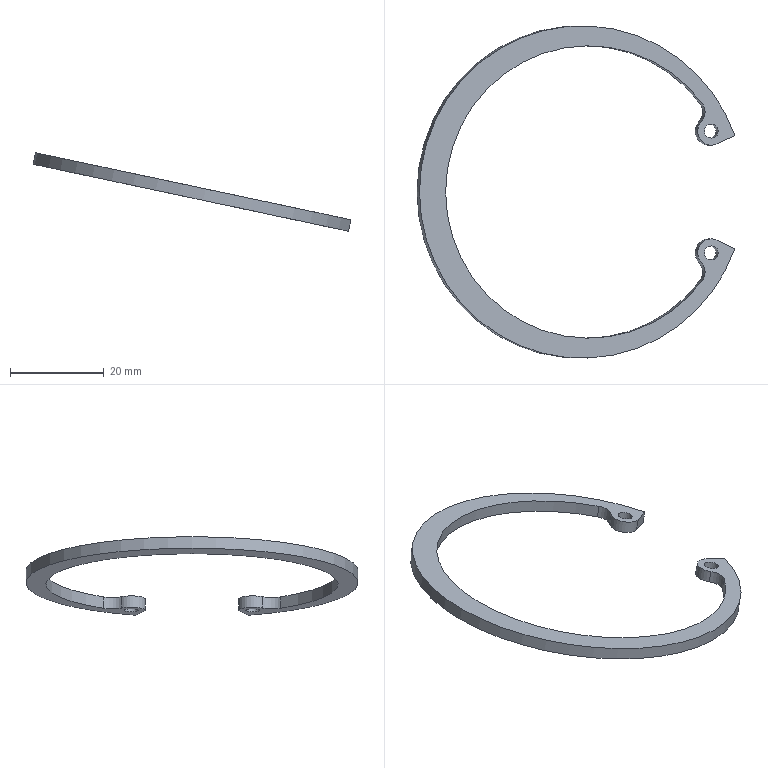Part | STEP file | HL4GZ-1.862.561 (elastic retaining ring -68) | 1 solid | 12 faces | box 67.9 x 71 x 16.767 mm | volume 2158 mm3 | cylinder 8 | plane 4 | commonest cylinder face diameters 6 x4 3 x2 62.45 x1 71 x1
STEP:
#1=CARTESIAN_POINT('',(0.,0.,0.));
#2=DIRECTION('',(0.,0.,1.));
#3=DIRECTION('',(1.,0.,0.));
#4=AXIS2_PLACEMENT_3D('',#1,#2,#3);
#5=CARTESIAN_POINT('',(2011.347,-82.992,-328.038));
#6=VERTEX_POINT('',#5);
#7=CARTESIAN_POINT('',(2011.347,-81.492,-328.038));
#8=DIRECTION('',(0.2079,0.,0.9781));
#9=DIRECTION('',(0.,1.,0.));
#10=AXIS2_PLACEMENT_3D('',#7,#8,#9);
#11=CIRCLE('',#10,1.5);
#12=CARTESIAN_POINT('',(1983.401,-94.424,-322.098));
#13=DIRECTION('',(-0.2079,0.,-0.9781));
#14=DIRECTION('',(0.,-1.,0.));
#15=AXIS2_PLACEMENT_3D('',#12,#13,#14);
#16=PLANE('',#15);
#17=CARTESIAN_POINT('',(-14.432,-28.571));
#18=CARTESIAN_POINT('',(-14.432,-25.973));
#19=CARTESIAN_POINT('',(-12.182,-27.272));
#20=CARTESIAN_POINT('',(-9.932,-28.571));
#21=CARTESIAN_POINT('',(-12.182,-29.87));
#22=CARTESIAN_POINT('',(-14.432,-31.169));
#23=CARTESIAN_POINT('',(-14.432,-28.571));
#24=(BOUNDED_CURVE()B_SPLINE_CURVE(2,(#17,#18,#19,#20,#21,#22,#23),.UNSPECIFIED.,.T.,.F.)B_SPLINE_CURVE_WITH_KNOTS((1,2,2,2,2,1),(-2.094,0.,2.094,4.189,6.283,8.378),.UNSPECIFIED.)CURVE()GEOMETRIC_REPRESENTATION_ITEM()RATIONAL_B_SPLINE_CURVE((1.,0.5,1.,0.5,1.,0.5,1.))REPRESENTATION_ITEM(''));
#25=(GEOMETRIC_REPRESENTATION_CONTEXT(2)PARAMETRIC_REPRESENTATION_CONTEXT()REPRESENTATION_CONTEXT('',''));
#26=DEFINITIONAL_REPRESENTATION('',(#24),#25);
#27=PCURVE('',#16,#26);
#28=CARTESIAN_POINT('',(2011.867,-81.492,-325.593));
#29=DIRECTION('',(-0.2079,0.,-0.9781));
#30=DIRECTION('',(0.,1.,0.));
#31=AXIS2_PLACEMENT_3D('',#28,#29,#30);
#32=CYLINDRICAL_SURFACE('',#31,1.5);
#33=CARTESIAN_POINT('',(12.566,2.5));
#34=DIRECTION('',(-1.,0.));
#35=VECTOR('',#34,1.);
#36=LINE('',#33,#35);
#37=(GEOMETRIC_REPRESENTATION_CONTEXT(2)PARAMETRIC_REPRESENTATION_CONTEXT()REPRESENTATION_CONTEXT('',''));
#38=DEFINITIONAL_REPRESENTATION('',(#36),#37);
#39=PCURVE('',#32,#38);
#40=SURFACE_CURVE('',#11,(#27,#39),.PCURVE_S1.);
#41=EDGE_CURVE('',#6,#6,#40,.T.);
#42=ORIENTED_EDGE('',*,*,#41,.T.);
#43=EDGE_LOOP('',(#42));
#44=FACE_BOUND('',#43,.T.);
#45=CARTESIAN_POINT('',(2011.347,-109.008,-328.038));
#46=VERTEX_POINT('',#45);
#47=CARTESIAN_POINT('',(2011.347,-107.508,-328.038));
#48=DIRECTION('',(0.2079,0.,0.9781));
#49=DIRECTION('',(0.,1.,0.));
#50=AXIS2_PLACEMENT_3D('',#47,#48,#49);
#51=CIRCLE('',#50,1.5);
#52=CARTESIAN_POINT('',(11.583,-28.571));
#53=CARTESIAN_POINT('',(11.583,-25.973));
#54=CARTESIAN_POINT('',(13.833,-27.272));
#55=CARTESIAN_POINT('',(16.083,-28.571));
#56=CARTESIAN_POINT('',(13.833,-29.87));
#57=CARTESIAN_POINT('',(11.583,-31.169));
#58=CARTESIAN_POINT('',(11.583,-28.571));
#59=(BOUNDED_CURVE()B_SPLINE_CURVE(2,(#52,#53,#54,#55,#56,#57,#58),.UNSPECIFIED.,.T.,.F.)B_SPLINE_CURVE_WITH_KNOTS((1,2,2,2,2,1),(-2.094,0.,2.094,4.189,6.283,8.378),.UNSPECIFIED.)CURVE()GEOMETRIC_REPRESENTATION_ITEM()RATIONAL_B_SPLINE_CURVE((1.,0.5,1.,0.5,1.,0.5,1.))REPRESENTATION_ITEM(''));
#60=(GEOMETRIC_REPRESENTATION_CONTEXT(2)PARAMETRIC_REPRESENTATION_CONTEXT()REPRESENTATION_CONTEXT('',''));
#61=DEFINITIONAL_REPRESENTATION('',(#59),#60);
#62=PCURVE('',#16,#61);
#63=CARTESIAN_POINT('',(2011.867,-107.508,-325.593));
#64=DIRECTION('',(-0.2079,0.,-0.9781));
#65=DIRECTION('',(0.,1.,0.));
#66=AXIS2_PLACEMENT_3D('',#63,#64,#65);
#67=CYLINDRICAL_SURFACE('',#66,1.5);
#68=CARTESIAN_POINT('',(12.566,2.5));
#69=DIRECTION('',(-1.,0.));
#70=VECTOR('',#69,1.);
#71=LINE('',#68,#70);
#72=(GEOMETRIC_REPRESENTATION_CONTEXT(2)PARAMETRIC_REPRESENTATION_CONTEXT()REPRESENTATION_CONTEXT('',''));
#73=DEFINITIONAL_REPRESENTATION('',(#71),#72);
#74=PCURVE('',#67,#73);
#75=SURFACE_CURVE('',#51,(#62,#74),.PCURVE_S1.);
#76=EDGE_CURVE('',#46,#46,#75,.T.);
#77=ORIENTED_EDGE('',*,*,#76,.T.);
#78=EDGE_LOOP('',(#77));
#79=FACE_BOUND('',#78,.T.);
#80=CARTESIAN_POINT('',(2009.399,-113.43,-327.624));
#81=VERTEX_POINT('',#80);
#82=CARTESIAN_POINT('',(2009.399,-75.57,-327.624));
#83=VERTEX_POINT('',#82);
#84=CARTESIAN_POINT('',(1985.109,-94.5,-322.461));
#85=DIRECTION('',(-0.2079,0.,-0.9781));
#86=DIRECTION('',(-0.7779,0.6062,0.1653));
#87=AXIS2_PLACEMENT_3D('',#84,#85,#86);
#88=CIRCLE('',#87,31.225);
#89=CARTESIAN_POINT('',(0.07559,-1.747));
#90=DIRECTION('',(-0.6062,0.7953));
#91=AXIS2_PLACEMENT_2D('',#89,#90);
#92=CIRCLE('',#91,31.225);
#93=(GEOMETRIC_REPRESENTATION_CONTEXT(2)PARAMETRIC_REPRESENTATION_CONTEXT()REPRESENTATION_CONTEXT('',''));
#94=DEFINITIONAL_REPRESENTATION('',(#92),#93);
#95=PCURVE('',#16,#94);
#96=CARTESIAN_POINT('',(1985.629,-94.5,-320.015));
#97=DIRECTION('',(-0.2079,0.,-0.9781));
#98=DIRECTION('',(-0.7779,0.6062,0.1653));
#99=AXIS2_PLACEMENT_3D('',#96,#97,#98);
#100=CYLINDRICAL_SURFACE('',#99,31.225);
#101=CARTESIAN_POINT('',(0.,2.5));
#102=DIRECTION('',(1.,0.));
#103=VECTOR('',#102,1.);
#104=LINE('',#101,#103);
#105=(GEOMETRIC_REPRESENTATION_CONTEXT(2)PARAMETRIC_REPRESENTATION_CONTEXT()REPRESENTATION_CONTEXT('',''));
#106=DEFINITIONAL_REPRESENTATION('',(#104),#105);
#107=PCURVE('',#100,#106);
#108=SURFACE_CURVE('',#88,(#95,#107),.PCURVE_S1.);
#109=EDGE_CURVE('',#81,#83,#108,.T.);
#110=ORIENTED_EDGE('',*,*,#109,.F.);
#111=CARTESIAN_POINT('',(2009.206,-109.56,-327.583));
#112=VERTEX_POINT('',#111);
#113=CARTESIAN_POINT('',(2007.065,-111.611,-327.128));
#114=DIRECTION('',(-0.2079,0.,-0.9781));
#115=DIRECTION('',(-0.7136,-0.6839,0.1517));
#116=AXIS2_PLACEMENT_3D('',#113,#114,#115);
#117=CIRCLE('',#116,3.);
#118=CARTESIAN_POINT('',(17.187,-24.193));
#119=DIRECTION('',(0.6839,0.7296));
#120=AXIS2_PLACEMENT_2D('',#118,#119);
#121=CIRCLE('',#120,3.);
#122=(GEOMETRIC_REPRESENTATION_CONTEXT(2)PARAMETRIC_REPRESENTATION_CONTEXT()REPRESENTATION_CONTEXT('',''));
#123=DEFINITIONAL_REPRESENTATION('',(#121),#122);
#124=PCURVE('',#16,#123);
#125=CARTESIAN_POINT('',(2007.585,-111.611,-324.682));
#126=DIRECTION('',(-0.2079,0.,-0.9781));
#127=DIRECTION('',(-0.7136,-0.6839,0.1517));
#128=AXIS2_PLACEMENT_3D('',#125,#126,#127);
#129=CYLINDRICAL_SURFACE('',#128,3.);
#130=CARTESIAN_POINT('',(0.,2.5));
#131=DIRECTION('',(1.,0.));
#132=VECTOR('',#131,1.);
#133=LINE('',#130,#132);
#134=(GEOMETRIC_REPRESENTATION_CONTEXT(2)PARAMETRIC_REPRESENTATION_CONTEXT()REPRESENTATION_CONTEXT('',''));
#135=DEFINITIONAL_REPRESENTATION('',(#133),#134);
#136=PCURVE('',#129,#135);
#137=SURFACE_CURVE('',#117,(#124,#136),.PCURVE_S1.);
#138=EDGE_CURVE('',#112,#81,#137,.T.);
#139=ORIENTED_EDGE('',*,*,#138,.F.);
#140=CARTESIAN_POINT('',(2012.574,-104.783,-328.299));
#141=VERTEX_POINT('',#140);
#142=CARTESIAN_POINT('',(2011.347,-107.508,-328.038));
#143=DIRECTION('',(0.2079,0.,0.9781));
#144=DIRECTION('',(-0.7136,-0.6839,0.1517));
#145=AXIS2_PLACEMENT_3D('',#142,#143,#144);
#146=CIRCLE('',#145,3.);
#147=CARTESIAN_POINT('',(15.135,-26.382));
#148=CARTESIAN_POINT('',(18.926,-29.936));
#149=CARTESIAN_POINT('',(13.953,-31.442));
#150=CARTESIAN_POINT('',(8.98,-32.948));
#151=CARTESIAN_POINT('',(10.162,-27.888));
#152=CARTESIAN_POINT('',(11.344,-22.828));
#153=CARTESIAN_POINT('',(15.135,-26.382));
#154=(BOUNDED_CURVE()B_SPLINE_CURVE(2,(#147,#148,#149,#150,#151,#152,#153),.UNSPECIFIED.,.T.,.F.)B_SPLINE_CURVE_WITH_KNOTS((1,2,2,2,2,1),(-2.094,0.,2.094,4.189,6.283,8.378),.UNSPECIFIED.)CURVE()GEOMETRIC_REPRESENTATION_ITEM()RATIONAL_B_SPLINE_CURVE((1.,0.5,1.,0.5,1.,0.5,1.))REPRESENTATION_ITEM(''));
#155=(GEOMETRIC_REPRESENTATION_CONTEXT(2)PARAMETRIC_REPRESENTATION_CONTEXT()REPRESENTATION_CONTEXT('',''));
#156=DEFINITIONAL_REPRESENTATION('',(#154),#155);
#157=PCURVE('',#16,#156);
#158=CARTESIAN_POINT('',(2011.867,-107.508,-325.593));
#159=DIRECTION('',(-0.2079,0.,-0.9781));
#160=DIRECTION('',(-0.7136,-0.6839,0.1517));
#161=AXIS2_PLACEMENT_3D('',#158,#159,#160);
#162=CYLINDRICAL_SURFACE('',#161,3.);
#163=CARTESIAN_POINT('',(6.283,2.5));
#164=DIRECTION('',(-1.,0.));
#165=VECTOR('',#164,1.);
#166=LINE('',#163,#165);
#167=(GEOMETRIC_REPRESENTATION_CONTEXT(2)PARAMETRIC_REPRESENTATION_CONTEXT()REPRESENTATION_CONTEXT('',''));
#168=DEFINITIONAL_REPRESENTATION('',(#166),#167);
#169=PCURVE('',#162,#168);
#170=SURFACE_CURVE('',#146,(#157,#169),.PCURVE_S1.);
#171=EDGE_CURVE('',#141,#112,#170,.T.);
#172=ORIENTED_EDGE('',*,*,#171,.F.);
#173=CARTESIAN_POINT('',(2016.371,-106.57,-329.106));
#174=VERTEX_POINT('',#173);
#175=CARTESIAN_POINT('',(2012.574,-104.783,-328.299));
#176=DIRECTION('',(-0.8885,0.4183,0.1889));
#177=VECTOR('',#176,1.);
#178=LINE('',#175,#177);
#179=CARTESIAN_POINT('',(10.358,-29.826));
#180=DIRECTION('',(-0.4183,0.9083));
#181=VECTOR('',#180,1.);
#182=LINE('',#179,#181);
#183=(GEOMETRIC_REPRESENTATION_CONTEXT(2)PARAMETRIC_REPRESENTATION_CONTEXT()REPRESENTATION_CONTEXT('',''));
#184=DEFINITIONAL_REPRESENTATION('',(#182),#183);
#185=PCURVE('',#16,#184);
#186=CARTESIAN_POINT('',(2016.891,-106.57,-326.66));
#187=DIRECTION('',(0.4091,0.9083,-0.08696));
#188=DIRECTION('',(-0.2079,0.,-0.9781));
#189=AXIS2_PLACEMENT_3D('',#186,#187,#188);
#190=PLANE('',#189);
#191=CARTESIAN_POINT('',(2.5,4.273));
#192=DIRECTION('',(0.,1.));
#193=VECTOR('',#192,1.);
#194=LINE('',#191,#193);
#195=(GEOMETRIC_REPRESENTATION_CONTEXT(2)PARAMETRIC_REPRESENTATION_CONTEXT()REPRESENTATION_CONTEXT('',''));
#196=DEFINITIONAL_REPRESENTATION('',(#194),#195);
#197=PCURVE('',#190,#196);
#198=SURFACE_CURVE('',#178,(#185,#197),.PCURVE_S1.);
#199=EDGE_CURVE('',#174,#141,#198,.T.);
#200=ORIENTED_EDGE('',*,*,#199,.F.);
#201=CARTESIAN_POINT('',(2016.371,-82.43,-329.106));
#202=VERTEX_POINT('',#201);
#203=CARTESIAN_POINT('',(1983.715,-94.5,-322.165));
#204=DIRECTION('',(0.2079,0.,0.9781));
#205=DIRECTION('',(0.9199,-0.34,-0.1955));
#206=AXIS2_PLACEMENT_3D('',#203,#204,#205);
#207=CIRCLE('',#206,35.5);
#208=CARTESIAN_POINT('',(12.146,-33.707));
#209=CARTESIAN_POINT('',(-45.679,-54.613));
#210=CARTESIAN_POINT('',(-34.872,5.918));
#211=CARTESIAN_POINT('',(-24.064,66.448));
#212=CARTESIAN_POINT('',(22.953,26.824));
#213=CARTESIAN_POINT('',(69.97,-12.801));
#214=CARTESIAN_POINT('',(12.146,-33.707));
#215=(BOUNDED_CURVE()B_SPLINE_CURVE(2,(#208,#209,#210,#211,#212,#213,#214),.UNSPECIFIED.,.T.,.F.)B_SPLINE_CURVE_WITH_KNOTS((1,2,2,2,2,1),(-2.094,0.,2.094,4.189,6.283,8.378),.UNSPECIFIED.)CURVE()GEOMETRIC_REPRESENTATION_ITEM()RATIONAL_B_SPLINE_CURVE((1.,0.5,1.,0.5,1.,0.5,1.))REPRESENTATION_ITEM(''));
#216=(GEOMETRIC_REPRESENTATION_CONTEXT(2)PARAMETRIC_REPRESENTATION_CONTEXT()REPRESENTATION_CONTEXT('',''));
#217=DEFINITIONAL_REPRESENTATION('',(#215),#216);
#218=PCURVE('',#16,#217);
#219=CARTESIAN_POINT('',(1984.235,-94.5,-319.719));
#220=DIRECTION('',(-0.2079,0.,-0.9781));
#221=DIRECTION('',(0.9199,-0.34,-0.1955));
#222=AXIS2_PLACEMENT_3D('',#219,#220,#221);
#223=CYLINDRICAL_SURFACE('',#222,35.5);
#224=CARTESIAN_POINT('',(6.283,2.5));
#225=DIRECTION('',(-1.,0.));
#226=VECTOR('',#225,1.);
#227=LINE('',#224,#226);
#228=(GEOMETRIC_REPRESENTATION_CONTEXT(2)PARAMETRIC_REPRESENTATION_CONTEXT()REPRESENTATION_CONTEXT('',''));
#229=DEFINITIONAL_REPRESENTATION('',(#227),#228);
#230=PCURVE('',#223,#229);
#231=SURFACE_CURVE('',#207,(#218,#230),.PCURVE_S1.);
#232=EDGE_CURVE('',#202,#174,#231,.T.);
#233=ORIENTED_EDGE('',*,*,#232,.F.);
#234=CARTESIAN_POINT('',(2012.574,-84.217,-328.299));
#235=VERTEX_POINT('',#234);
#236=CARTESIAN_POINT('',(2016.371,-82.43,-329.106));
#237=DIRECTION('',(0.8885,0.4183,-0.1889));
#238=VECTOR('',#237,1.);
#239=LINE('',#236,#238);
#240=CARTESIAN_POINT('',(-11.994,-33.707));
#241=DIRECTION('',(-0.4183,-0.9083));
#242=VECTOR('',#241,1.);
#243=LINE('',#240,#242);
#244=(GEOMETRIC_REPRESENTATION_CONTEXT(2)PARAMETRIC_REPRESENTATION_CONTEXT()REPRESENTATION_CONTEXT('',''));
#245=DEFINITIONAL_REPRESENTATION('',(#243),#244);
#246=PCURVE('',#16,#245);
#247=CARTESIAN_POINT('',(2013.094,-84.217,-325.853));
#248=DIRECTION('',(0.4091,-0.9083,-0.08696));
#249=DIRECTION('',(0.2079,0.,0.9781));
#250=AXIS2_PLACEMENT_3D('',#247,#248,#249);
#251=PLANE('',#250);
#252=CARTESIAN_POINT('',(-2.5,-4.273));
#253=DIRECTION('',(0.,-1.));
#254=VECTOR('',#253,1.);
#255=LINE('',#252,#254);
#256=(GEOMETRIC_REPRESENTATION_CONTEXT(2)PARAMETRIC_REPRESENTATION_CONTEXT()REPRESENTATION_CONTEXT('',''));
#257=DEFINITIONAL_REPRESENTATION('',(#255),#256);
#258=PCURVE('',#251,#257);
#259=SURFACE_CURVE('',#239,(#246,#258),.PCURVE_S1.);
#260=EDGE_CURVE('',#235,#202,#259,.T.);
#261=ORIENTED_EDGE('',*,*,#260,.F.);
#262=CARTESIAN_POINT('',(2009.206,-79.44,-327.583));
#263=VERTEX_POINT('',#262);
#264=CARTESIAN_POINT('',(2011.347,-81.492,-328.038));
#265=DIRECTION('',(0.2079,0.,0.9781));
#266=DIRECTION('',(0.4091,-0.9083,-0.08696));
#267=AXIS2_PLACEMENT_3D('',#264,#265,#266);
#268=CIRCLE('',#267,3.);
#269=CARTESIAN_POINT('',(-10.207,-29.826));
#270=CARTESIAN_POINT('',(-12.381,-34.545));
#271=CARTESIAN_POINT('',(-15.381,-30.303));
#272=CARTESIAN_POINT('',(-18.382,-26.061));
#273=CARTESIAN_POINT('',(-13.208,-25.583));
#274=CARTESIAN_POINT('',(-8.034,-25.106));
#275=CARTESIAN_POINT('',(-10.207,-29.826));
#276=(BOUNDED_CURVE()B_SPLINE_CURVE(2,(#269,#270,#271,#272,#273,#274,#275),.UNSPECIFIED.,.T.,.F.)B_SPLINE_CURVE_WITH_KNOTS((1,2,2,2,2,1),(-2.094,0.,2.094,4.189,6.283,8.378),.UNSPECIFIED.)CURVE()GEOMETRIC_REPRESENTATION_ITEM()RATIONAL_B_SPLINE_CURVE((1.,0.5,1.,0.5,1.,0.5,1.))REPRESENTATION_ITEM(''));
#277=(GEOMETRIC_REPRESENTATION_CONTEXT(2)PARAMETRIC_REPRESENTATION_CONTEXT()REPRESENTATION_CONTEXT('',''));
#278=DEFINITIONAL_REPRESENTATION('',(#276),#277);
#279=PCURVE('',#16,#278);
#280=CARTESIAN_POINT('',(2011.867,-81.492,-325.593));
#281=DIRECTION('',(-0.2079,0.,-0.9781));
#282=DIRECTION('',(0.4091,-0.9083,-0.08696));
#283=AXIS2_PLACEMENT_3D('',#280,#281,#282);
#284=CYLINDRICAL_SURFACE('',#283,3.);
#285=CARTESIAN_POINT('',(6.283,2.5));
#286=DIRECTION('',(-1.,0.));
#287=VECTOR('',#286,1.);
#288=LINE('',#285,#287);
#289=(GEOMETRIC_REPRESENTATION_CONTEXT(2)PARAMETRIC_REPRESENTATION_CONTEXT()REPRESENTATION_CONTEXT('',''));
#290=DEFINITIONAL_REPRESENTATION('',(#288),#289);
#291=PCURVE('',#284,#290);
#292=SURFACE_CURVE('',#268,(#279,#291),.PCURVE_S1.);
#293=EDGE_CURVE('',#263,#235,#292,.T.);
#294=ORIENTED_EDGE('',*,*,#293,.F.);
#295=CARTESIAN_POINT('',(2007.065,-77.389,-327.128));
#296=DIRECTION('',(-0.2079,0.,-0.9781));
#297=DIRECTION('',(-0.7779,-0.6062,0.1653));
#298=AXIS2_PLACEMENT_3D('',#295,#296,#297);
#299=CIRCLE('',#298,3.);
#300=CARTESIAN_POINT('',(-17.036,-24.193));
#301=DIRECTION('',(0.6062,0.7953));
#302=AXIS2_PLACEMENT_2D('',#300,#301);
#303=CIRCLE('',#302,3.);
#304=(GEOMETRIC_REPRESENTATION_CONTEXT(2)PARAMETRIC_REPRESENTATION_CONTEXT()REPRESENTATION_CONTEXT('',''));
#305=DEFINITIONAL_REPRESENTATION('',(#303),#304);
#306=PCURVE('',#16,#305);
#307=CARTESIAN_POINT('',(2007.585,-77.389,-324.682));
#308=DIRECTION('',(-0.2079,0.,-0.9781));
#309=DIRECTION('',(-0.7779,-0.6062,0.1653));
#310=AXIS2_PLACEMENT_3D('',#307,#308,#309);
#311=CYLINDRICAL_SURFACE('',#310,3.);
#312=CARTESIAN_POINT('',(0.,2.5));
#313=DIRECTION('',(1.,0.));
#314=VECTOR('',#313,1.);
#315=LINE('',#312,#314);
#316=(GEOMETRIC_REPRESENTATION_CONTEXT(2)PARAMETRIC_REPRESENTATION_CONTEXT()REPRESENTATION_CONTEXT('',''));
#317=DEFINITIONAL_REPRESENTATION('',(#315),#316);
#318=PCURVE('',#311,#317);
#319=SURFACE_CURVE('',#299,(#306,#318),.PCURVE_S1.);
#320=EDGE_CURVE('',#83,#263,#319,.T.);
#321=ORIENTED_EDGE('',*,*,#320,.F.);
#322=EDGE_LOOP('',(#110,#139,#172,#200,#233,#261,#294,#321));
#323=FACE_BOUND('',#322,.T.);
#324=ADVANCED_FACE('',(#44,#79,#323),#16,.T.);
#325=CARTESIAN_POINT('',(2011.867,-82.992,-325.593));
#326=VERTEX_POINT('',#325);
#327=CARTESIAN_POINT('',(2011.867,-81.492,-325.593));
#328=DIRECTION('',(-0.2079,0.,-0.9781));
#329=DIRECTION('',(0.,1.,0.));
#330=AXIS2_PLACEMENT_3D('',#327,#328,#329);
#331=CIRCLE('',#330,1.5);
#332=CARTESIAN_POINT('',(1983.92,-94.424,-319.652));
#333=DIRECTION('',(-0.2079,0.,-0.9781));
#334=DIRECTION('',(0.,-1.,0.));
#335=AXIS2_PLACEMENT_3D('',#332,#333,#334);
#336=PLANE('',#335);
#337=CARTESIAN_POINT('',(-12.932,-28.571));
#338=DIRECTION('',(-1.,0.));
#339=AXIS2_PLACEMENT_2D('',#337,#338);
#340=CIRCLE('',#339,1.5);
#341=(GEOMETRIC_REPRESENTATION_CONTEXT(2)PARAMETRIC_REPRESENTATION_CONTEXT()REPRESENTATION_CONTEXT('',''));
#342=DEFINITIONAL_REPRESENTATION('',(#340),#341);
#343=PCURVE('',#336,#342);
#344=CARTESIAN_POINT('',(0.,0.));
#345=DIRECTION('',(1.,0.));
#346=VECTOR('',#345,1.);
#347=LINE('',#344,#346);
#348=(GEOMETRIC_REPRESENTATION_CONTEXT(2)PARAMETRIC_REPRESENTATION_CONTEXT()REPRESENTATION_CONTEXT('',''));
#349=DEFINITIONAL_REPRESENTATION('',(#347),#348);
#350=PCURVE('',#32,#349);
#351=SURFACE_CURVE('',#331,(#343,#350),.PCURVE_S1.);
#352=EDGE_CURVE('',#326,#326,#351,.T.);
#353=ORIENTED_EDGE('',*,*,#352,.T.);
#354=EDGE_LOOP('',(#353));
#355=FACE_BOUND('',#354,.T.);
#356=CARTESIAN_POINT('',(2011.867,-109.008,-325.593));
#357=VERTEX_POINT('',#356);
#358=CARTESIAN_POINT('',(2011.867,-107.508,-325.593));
#359=DIRECTION('',(-0.2079,0.,-0.9781));
#360=DIRECTION('',(0.,1.,0.));
#361=AXIS2_PLACEMENT_3D('',#358,#359,#360);
#362=CIRCLE('',#361,1.5);
#363=CARTESIAN_POINT('',(13.083,-28.571));
#364=DIRECTION('',(-1.,0.));
#365=AXIS2_PLACEMENT_2D('',#363,#364);
#366=CIRCLE('',#365,1.5);
#367=(GEOMETRIC_REPRESENTATION_CONTEXT(2)PARAMETRIC_REPRESENTATION_CONTEXT()REPRESENTATION_CONTEXT('',''));
#368=DEFINITIONAL_REPRESENTATION('',(#366),#367);
#369=PCURVE('',#336,#368);
#370=CARTESIAN_POINT('',(0.,0.));
#371=DIRECTION('',(1.,0.));
#372=VECTOR('',#371,1.);
#373=LINE('',#370,#372);
#374=(GEOMETRIC_REPRESENTATION_CONTEXT(2)PARAMETRIC_REPRESENTATION_CONTEXT()REPRESENTATION_CONTEXT('',''));
#375=DEFINITIONAL_REPRESENTATION('',(#373),#374);
#376=PCURVE('',#67,#375);
#377=SURFACE_CURVE('',#362,(#369,#376),.PCURVE_S1.);
#378=EDGE_CURVE('',#357,#357,#377,.T.);
#379=ORIENTED_EDGE('',*,*,#378,.T.);
#380=EDGE_LOOP('',(#379));
#381=FACE_BOUND('',#380,.T.);
#382=CARTESIAN_POINT('',(2009.919,-75.57,-325.178));
#383=VERTEX_POINT('',#382);
#384=CARTESIAN_POINT('',(2009.919,-113.43,-325.178));
#385=VERTEX_POINT('',#384);
#386=CARTESIAN_POINT('',(1985.629,-94.5,-320.015));
#387=DIRECTION('',(0.2079,0.,0.9781));
#388=DIRECTION('',(-0.7779,0.6062,0.1653));
#389=AXIS2_PLACEMENT_3D('',#386,#387,#388);
#390=CIRCLE('',#389,31.225);
#391=CARTESIAN_POINT('',(-18.854,23.086));
#392=CARTESIAN_POINT('',(24.157,55.874));
#393=CARTESIAN_POINT('',(31.046,2.231));
#394=CARTESIAN_POINT('',(37.936,-51.412));
#395=CARTESIAN_POINT('',(-11.965,-30.557));
#396=CARTESIAN_POINT('',(-61.866,-9.702));
#397=CARTESIAN_POINT('',(-18.854,23.086));
#398=(BOUNDED_CURVE()B_SPLINE_CURVE(2,(#391,#392,#393,#394,#395,#396,#397),.UNSPECIFIED.,.T.,.F.)B_SPLINE_CURVE_WITH_KNOTS((1,2,2,2,2,1),(-2.094,0.,2.094,4.189,6.283,8.378),.UNSPECIFIED.)CURVE()GEOMETRIC_REPRESENTATION_ITEM()RATIONAL_B_SPLINE_CURVE((1.,0.5,1.,0.5,1.,0.5,1.))REPRESENTATION_ITEM(''));
#399=(GEOMETRIC_REPRESENTATION_CONTEXT(2)PARAMETRIC_REPRESENTATION_CONTEXT()REPRESENTATION_CONTEXT('',''));
#400=DEFINITIONAL_REPRESENTATION('',(#398),#399);
#401=PCURVE('',#336,#400);
#402=CARTESIAN_POINT('',(12.566,0.));
#403=DIRECTION('',(-1.,0.));
#404=VECTOR('',#403,1.);
#405=LINE('',#402,#404);
#406=(GEOMETRIC_REPRESENTATION_CONTEXT(2)PARAMETRIC_REPRESENTATION_CONTEXT()REPRESENTATION_CONTEXT('',''));
#407=DEFINITIONAL_REPRESENTATION('',(#405),#406);
#408=PCURVE('',#100,#407);
#409=SURFACE_CURVE('',#390,(#401,#408),.PCURVE_S1.);
#410=EDGE_CURVE('',#383,#385,#409,.T.);
#411=ORIENTED_EDGE('',*,*,#410,.F.);
#412=CARTESIAN_POINT('',(2009.726,-79.44,-325.137));
#413=VERTEX_POINT('',#412);
#414=CARTESIAN_POINT('',(2007.585,-77.389,-324.682));
#415=DIRECTION('',(0.2079,0.,0.9781));
#416=DIRECTION('',(-0.7779,-0.6062,0.1653));
#417=AXIS2_PLACEMENT_3D('',#414,#415,#416);
#418=CIRCLE('',#417,3.);
#419=CARTESIAN_POINT('',(-15.217,-21.808));
#420=CARTESIAN_POINT('',(-11.085,-24.958));
#421=CARTESIAN_POINT('',(-15.879,-26.961));
#422=CARTESIAN_POINT('',(-20.673,-28.965));
#423=CARTESIAN_POINT('',(-20.011,-23.811));
#424=CARTESIAN_POINT('',(-19.349,-18.657));
#425=CARTESIAN_POINT('',(-15.217,-21.808));
#426=(BOUNDED_CURVE()B_SPLINE_CURVE(2,(#419,#420,#421,#422,#423,#424,#425),.UNSPECIFIED.,.T.,.F.)B_SPLINE_CURVE_WITH_KNOTS((1,2,2,2,2,1),(-2.094,0.,2.094,4.189,6.283,8.378),.UNSPECIFIED.)CURVE()GEOMETRIC_REPRESENTATION_ITEM()RATIONAL_B_SPLINE_CURVE((1.,0.5,1.,0.5,1.,0.5,1.))REPRESENTATION_ITEM(''));
#427=(GEOMETRIC_REPRESENTATION_CONTEXT(2)PARAMETRIC_REPRESENTATION_CONTEXT()REPRESENTATION_CONTEXT('',''));
#428=DEFINITIONAL_REPRESENTATION('',(#426),#427);
#429=PCURVE('',#336,#428);
#430=CARTESIAN_POINT('',(6.283,0.));
#431=DIRECTION('',(-1.,0.));
#432=VECTOR('',#431,1.);
#433=LINE('',#430,#432);
#434=(GEOMETRIC_REPRESENTATION_CONTEXT(2)PARAMETRIC_REPRESENTATION_CONTEXT()REPRESENTATION_CONTEXT('',''));
#435=DEFINITIONAL_REPRESENTATION('',(#433),#434);
#436=PCURVE('',#311,#435);
#437=SURFACE_CURVE('',#418,(#429,#436),.PCURVE_S1.);
#438=EDGE_CURVE('',#413,#383,#437,.T.);
#439=ORIENTED_EDGE('',*,*,#438,.F.);
#440=CARTESIAN_POINT('',(2013.094,-84.217,-325.853));
#441=VERTEX_POINT('',#440);
#442=CARTESIAN_POINT('',(2011.867,-81.492,-325.593));
#443=DIRECTION('',(-0.2079,0.,-0.9781));
#444=DIRECTION('',(0.4091,-0.9083,-0.08696));
#445=AXIS2_PLACEMENT_3D('',#442,#443,#444);
#446=CIRCLE('',#445,3.);
#447=CARTESIAN_POINT('',(-12.932,-28.571));
#448=DIRECTION('',(0.9083,-0.4183));
#449=AXIS2_PLACEMENT_2D('',#447,#448);
#450=CIRCLE('',#449,3.);
#451=(GEOMETRIC_REPRESENTATION_CONTEXT(2)PARAMETRIC_REPRESENTATION_CONTEXT()REPRESENTATION_CONTEXT('',''));
#452=DEFINITIONAL_REPRESENTATION('',(#450),#451);
#453=PCURVE('',#336,#452);
#454=CARTESIAN_POINT('',(0.,0.));
#455=DIRECTION('',(1.,0.));
#456=VECTOR('',#455,1.);
#457=LINE('',#454,#456);
#458=(GEOMETRIC_REPRESENTATION_CONTEXT(2)PARAMETRIC_REPRESENTATION_CONTEXT()REPRESENTATION_CONTEXT('',''));
#459=DEFINITIONAL_REPRESENTATION('',(#457),#458);
#460=PCURVE('',#284,#459);
#461=SURFACE_CURVE('',#446,(#453,#460),.PCURVE_S1.);
#462=EDGE_CURVE('',#441,#413,#461,.T.);
#463=ORIENTED_EDGE('',*,*,#462,.F.);
#464=CARTESIAN_POINT('',(2016.891,-82.43,-326.66));
#465=VERTEX_POINT('',#464);
#466=CARTESIAN_POINT('',(2016.891,-82.43,-326.66));
#467=DIRECTION('',(-0.8885,-0.4183,0.1889));
#468=VECTOR('',#467,1.);
#469=LINE('',#466,#468);
#470=CARTESIAN_POINT('',(-11.994,-33.707));
#471=DIRECTION('',(0.4183,0.9083));
#472=VECTOR('',#471,1.);
#473=LINE('',#470,#472);
#474=(GEOMETRIC_REPRESENTATION_CONTEXT(2)PARAMETRIC_REPRESENTATION_CONTEXT()REPRESENTATION_CONTEXT('',''));
#475=DEFINITIONAL_REPRESENTATION('',(#473),#474);
#476=PCURVE('',#336,#475);
#477=CARTESIAN_POINT('',(0.,-4.273));
#478=DIRECTION('',(0.,1.));
#479=VECTOR('',#478,1.);
#480=LINE('',#477,#479);
#481=(GEOMETRIC_REPRESENTATION_CONTEXT(2)PARAMETRIC_REPRESENTATION_CONTEXT()REPRESENTATION_CONTEXT('',''));
#482=DEFINITIONAL_REPRESENTATION('',(#480),#481);
#483=PCURVE('',#251,#482);
#484=SURFACE_CURVE('',#469,(#476,#483),.PCURVE_S1.);
#485=EDGE_CURVE('',#465,#441,#484,.T.);
#486=ORIENTED_EDGE('',*,*,#485,.F.);
#487=CARTESIAN_POINT('',(2016.891,-106.57,-326.66));
#488=VERTEX_POINT('',#487);
#489=CARTESIAN_POINT('',(1984.235,-94.5,-319.719));
#490=DIRECTION('',(-0.2079,0.,-0.9781));
#491=DIRECTION('',(0.9199,-0.34,-0.1955));
#492=AXIS2_PLACEMENT_3D('',#489,#490,#491);
#493=CIRCLE('',#492,35.5);
#494=CARTESIAN_POINT('',(0.07559,-0.3217));
#495=DIRECTION('',(0.34,-0.9404));
#496=AXIS2_PLACEMENT_2D('',#494,#495);
#497=CIRCLE('',#496,35.5);
#498=(GEOMETRIC_REPRESENTATION_CONTEXT(2)PARAMETRIC_REPRESENTATION_CONTEXT()REPRESENTATION_CONTEXT('',''));
#499=DEFINITIONAL_REPRESENTATION('',(#497),#498);
#500=PCURVE('',#336,#499);
#501=CARTESIAN_POINT('',(0.,0.));
#502=DIRECTION('',(1.,0.));
#503=VECTOR('',#502,1.);
#504=LINE('',#501,#503);
#505=(GEOMETRIC_REPRESENTATION_CONTEXT(2)PARAMETRIC_REPRESENTATION_CONTEXT()REPRESENTATION_CONTEXT('',''));
#506=DEFINITIONAL_REPRESENTATION('',(#504),#505);
#507=PCURVE('',#223,#506);
#508=SURFACE_CURVE('',#493,(#500,#507),.PCURVE_S1.);
#509=EDGE_CURVE('',#488,#465,#508,.T.);
#510=ORIENTED_EDGE('',*,*,#509,.F.);
#511=CARTESIAN_POINT('',(2013.094,-104.783,-325.853));
#512=VERTEX_POINT('',#511);
#513=CARTESIAN_POINT('',(2013.094,-104.783,-325.853));
#514=DIRECTION('',(0.8885,-0.4183,-0.1889));
#515=VECTOR('',#514,1.);
#516=LINE('',#513,#515);
#517=CARTESIAN_POINT('',(10.358,-29.826));
#518=DIRECTION('',(0.4183,-0.9083));
#519=VECTOR('',#518,1.);
#520=LINE('',#517,#519);
#521=(GEOMETRIC_REPRESENTATION_CONTEXT(2)PARAMETRIC_REPRESENTATION_CONTEXT()REPRESENTATION_CONTEXT('',''));
#522=DEFINITIONAL_REPRESENTATION('',(#520),#521);
#523=PCURVE('',#336,#522);
#524=CARTESIAN_POINT('',(0.,4.273));
#525=DIRECTION('',(0.,-1.));
#526=VECTOR('',#525,1.);
#527=LINE('',#524,#526);
#528=(GEOMETRIC_REPRESENTATION_CONTEXT(2)PARAMETRIC_REPRESENTATION_CONTEXT()REPRESENTATION_CONTEXT('',''));
#529=DEFINITIONAL_REPRESENTATION('',(#527),#528);
#530=PCURVE('',#190,#529);
#531=SURFACE_CURVE('',#516,(#523,#530),.PCURVE_S1.);
#532=EDGE_CURVE('',#512,#488,#531,.T.);
#533=ORIENTED_EDGE('',*,*,#532,.F.);
#534=CARTESIAN_POINT('',(2009.726,-109.56,-325.137));
#535=VERTEX_POINT('',#534);
#536=CARTESIAN_POINT('',(2011.867,-107.508,-325.593));
#537=DIRECTION('',(-0.2079,0.,-0.9781));
#538=DIRECTION('',(-0.7136,-0.6839,0.1517));
#539=AXIS2_PLACEMENT_3D('',#536,#537,#538);
#540=CIRCLE('',#539,3.);
#541=CARTESIAN_POINT('',(13.083,-28.571));
#542=DIRECTION('',(0.6839,0.7296));
#543=AXIS2_PLACEMENT_2D('',#541,#542);
#544=CIRCLE('',#543,3.);
#545=(GEOMETRIC_REPRESENTATION_CONTEXT(2)PARAMETRIC_REPRESENTATION_CONTEXT()REPRESENTATION_CONTEXT('',''));
#546=DEFINITIONAL_REPRESENTATION('',(#544),#545);
#547=PCURVE('',#336,#546);
#548=CARTESIAN_POINT('',(0.,0.));
#549=DIRECTION('',(1.,0.));
#550=VECTOR('',#549,1.);
#551=LINE('',#548,#550);
#552=(GEOMETRIC_REPRESENTATION_CONTEXT(2)PARAMETRIC_REPRESENTATION_CONTEXT()REPRESENTATION_CONTEXT('',''));
#553=DEFINITIONAL_REPRESENTATION('',(#551),#552);
#554=PCURVE('',#162,#553);
#555=SURFACE_CURVE('',#540,(#547,#554),.PCURVE_S1.);
#556=EDGE_CURVE('',#535,#512,#555,.T.);
#557=ORIENTED_EDGE('',*,*,#556,.F.);
#558=CARTESIAN_POINT('',(2007.585,-111.611,-324.682));
#559=DIRECTION('',(0.2079,0.,0.9781));
#560=DIRECTION('',(-0.7136,-0.6839,0.1517));
#561=AXIS2_PLACEMENT_3D('',#558,#559,#560);
#562=CIRCLE('',#561,3.);
#563=CARTESIAN_POINT('',(19.239,-22.005));
#564=CARTESIAN_POINT('',(23.03,-25.559));
#565=CARTESIAN_POINT('',(18.056,-27.065));
#566=CARTESIAN_POINT('',(13.083,-28.571));
#567=CARTESIAN_POINT('',(14.266,-23.511));
#568=CARTESIAN_POINT('',(15.448,-18.451));
#569=CARTESIAN_POINT('',(19.239,-22.005));
#570=(BOUNDED_CURVE()B_SPLINE_CURVE(2,(#563,#564,#565,#566,#567,#568,#569),.UNSPECIFIED.,.T.,.F.)B_SPLINE_CURVE_WITH_KNOTS((1,2,2,2,2,1),(-2.094,0.,2.094,4.189,6.283,8.378),.UNSPECIFIED.)CURVE()GEOMETRIC_REPRESENTATION_ITEM()RATIONAL_B_SPLINE_CURVE((1.,0.5,1.,0.5,1.,0.5,1.))REPRESENTATION_ITEM(''));
#571=(GEOMETRIC_REPRESENTATION_CONTEXT(2)PARAMETRIC_REPRESENTATION_CONTEXT()REPRESENTATION_CONTEXT('',''));
#572=DEFINITIONAL_REPRESENTATION('',(#570),#571);
#573=PCURVE('',#336,#572);
#574=CARTESIAN_POINT('',(6.283,0.));
#575=DIRECTION('',(-1.,0.));
#576=VECTOR('',#575,1.);
#577=LINE('',#574,#576);
#578=(GEOMETRIC_REPRESENTATION_CONTEXT(2)PARAMETRIC_REPRESENTATION_CONTEXT()REPRESENTATION_CONTEXT('',''));
#579=DEFINITIONAL_REPRESENTATION('',(#577),#578);
#580=PCURVE('',#129,#579);
#581=SURFACE_CURVE('',#562,(#573,#580),.PCURVE_S1.);
#582=EDGE_CURVE('',#385,#535,#581,.T.);
#583=ORIENTED_EDGE('',*,*,#582,.F.);
#584=EDGE_LOOP('',(#411,#439,#463,#486,#510,#533,#557,#583));
#585=FACE_BOUND('',#584,.T.);
#586=ADVANCED_FACE('',(#355,#381,#585),#336,.F.);
#587=CARTESIAN_POINT('',(2009.726,-109.56,-325.137));
#588=DIRECTION('',(-0.2079,0.,-0.9781));
#589=VECTOR('',#588,1.);
#590=LINE('',#587,#589);
#591=CARTESIAN_POINT('',(3.142,0.));
#592=DIRECTION('',(0.,1.));
#593=VECTOR('',#592,1.);
#594=LINE('',#591,#593);
#595=(GEOMETRIC_REPRESENTATION_CONTEXT(2)PARAMETRIC_REPRESENTATION_CONTEXT()REPRESENTATION_CONTEXT('',''));
#596=DEFINITIONAL_REPRESENTATION('',(#594),#595);
#597=PCURVE('',#129,#596);
#598=CARTESIAN_POINT('',(0.,0.));
#599=DIRECTION('',(0.,1.));
#600=VECTOR('',#599,1.);
#601=LINE('',#598,#600);
#602=(GEOMETRIC_REPRESENTATION_CONTEXT(2)PARAMETRIC_REPRESENTATION_CONTEXT()REPRESENTATION_CONTEXT('',''));
#603=DEFINITIONAL_REPRESENTATION('',(#601),#602);
#604=PCURVE('',#162,#603);
#605=SURFACE_CURVE('',#590,(#597,#604),.PCURVE_S1.);
#606=EDGE_CURVE('',#535,#112,#605,.T.);
#607=ORIENTED_EDGE('',*,*,#606,.F.);
#608=ORIENTED_EDGE('',*,*,#582,.F.);
#609=CARTESIAN_POINT('',(2009.919,-113.43,-325.178));
#610=DIRECTION('',(-0.2079,0.,-0.9781));
#611=VECTOR('',#610,1.);
#612=LINE('',#609,#611);
#613=CARTESIAN_POINT('',(4.546,0.));
#614=DIRECTION('',(0.,1.));
#615=VECTOR('',#614,1.);
#616=LINE('',#613,#615);
#617=(GEOMETRIC_REPRESENTATION_CONTEXT(2)PARAMETRIC_REPRESENTATION_CONTEXT()REPRESENTATION_CONTEXT('',''));
#618=DEFINITIONAL_REPRESENTATION('',(#616),#617);
#619=PCURVE('',#129,#618);
#620=CARTESIAN_POINT('',(3.142,0.));
#621=DIRECTION('',(0.,1.));
#622=VECTOR('',#621,1.);
#623=LINE('',#620,#622);
#624=(GEOMETRIC_REPRESENTATION_CONTEXT(2)PARAMETRIC_REPRESENTATION_CONTEXT()REPRESENTATION_CONTEXT('',''));
#625=DEFINITIONAL_REPRESENTATION('',(#623),#624);
#626=PCURVE('',#100,#625);
#627=SURFACE_CURVE('',#612,(#619,#626),.PCURVE_S1.);
#628=EDGE_CURVE('',#385,#81,#627,.T.);
#629=ORIENTED_EDGE('',*,*,#628,.T.);
#630=ORIENTED_EDGE('',*,*,#138,.F.);
#631=EDGE_LOOP('',(#607,#608,#629,#630));
#632=FACE_BOUND('',#631,.F.);
#633=ADVANCED_FACE('',(#632),#129,.F.);
#634=ORIENTED_EDGE('',*,*,#171,.T.);
#635=ORIENTED_EDGE('',*,*,#606,.F.);
#636=ORIENTED_EDGE('',*,*,#556,.T.);
#637=CARTESIAN_POINT('',(2013.094,-104.783,-325.853));
#638=DIRECTION('',(-0.2079,0.,-0.9781));
#639=VECTOR('',#638,1.);
#640=LINE('',#637,#639);
#641=CARTESIAN_POINT('',(2.755,0.));
#642=DIRECTION('',(0.,1.));
#643=VECTOR('',#642,1.);
#644=LINE('',#641,#643);
#645=(GEOMETRIC_REPRESENTATION_CONTEXT(2)PARAMETRIC_REPRESENTATION_CONTEXT()REPRESENTATION_CONTEXT('',''));
#646=DEFINITIONAL_REPRESENTATION('',(#644),#645);
#647=PCURVE('',#162,#646);
#648=CARTESIAN_POINT('',(0.,4.273));
#649=DIRECTION('',(1.,0.));
#650=VECTOR('',#649,1.);
#651=LINE('',#648,#650);
#652=(GEOMETRIC_REPRESENTATION_CONTEXT(2)PARAMETRIC_REPRESENTATION_CONTEXT()REPRESENTATION_CONTEXT('',''));
#653=DEFINITIONAL_REPRESENTATION('',(#651),#652);
#654=PCURVE('',#190,#653);
#655=SURFACE_CURVE('',#640,(#647,#654),.PCURVE_S1.);
#656=EDGE_CURVE('',#512,#141,#655,.T.);
#657=ORIENTED_EDGE('',*,*,#656,.T.);
#658=EDGE_LOOP('',(#634,#635,#636,#657));
#659=FACE_BOUND('',#658,.T.);
#660=ADVANCED_FACE('',(#659),#162,.T.);
#661=ORIENTED_EDGE('',*,*,#199,.T.);
#662=ORIENTED_EDGE('',*,*,#656,.F.);
#663=ORIENTED_EDGE('',*,*,#532,.T.);
#664=CARTESIAN_POINT('',(2016.891,-106.57,-326.66));
#665=DIRECTION('',(-0.2079,0.,-0.9781));
#666=VECTOR('',#665,1.);
#667=LINE('',#664,#666);
#668=CARTESIAN_POINT('',(0.,0.));
#669=DIRECTION('',(1.,0.));
#670=VECTOR('',#669,1.);
#671=LINE('',#668,#670);
#672=(GEOMETRIC_REPRESENTATION_CONTEXT(2)PARAMETRIC_REPRESENTATION_CONTEXT()REPRESENTATION_CONTEXT('',''));
#673=DEFINITIONAL_REPRESENTATION('',(#671),#672);
#674=PCURVE('',#190,#673);
#675=CARTESIAN_POINT('',(0.,0.));
#676=DIRECTION('',(0.,1.));
#677=VECTOR('',#676,1.);
#678=LINE('',#675,#677);
#679=(GEOMETRIC_REPRESENTATION_CONTEXT(2)PARAMETRIC_REPRESENTATION_CONTEXT()REPRESENTATION_CONTEXT('',''));
#680=DEFINITIONAL_REPRESENTATION('',(#678),#679);
#681=PCURVE('',#223,#680);
#682=SURFACE_CURVE('',#667,(#674,#681),.PCURVE_S1.);
#683=EDGE_CURVE('',#488,#174,#682,.T.);
#684=ORIENTED_EDGE('',*,*,#683,.T.);
#685=EDGE_LOOP('',(#661,#662,#663,#684));
#686=FACE_BOUND('',#685,.T.);
#687=ADVANCED_FACE('',(#686),#190,.T.);
#688=ORIENTED_EDGE('',*,*,#232,.T.);
#689=ORIENTED_EDGE('',*,*,#683,.F.);
#690=ORIENTED_EDGE('',*,*,#509,.T.);
#691=CARTESIAN_POINT('',(2016.891,-82.43,-326.66));
#692=DIRECTION('',(-0.2079,0.,-0.9781));
#693=VECTOR('',#692,1.);
#694=LINE('',#691,#693);
#695=CARTESIAN_POINT('',(5.589,0.));
#696=DIRECTION('',(0.,1.));
#697=VECTOR('',#696,1.);
#698=LINE('',#695,#697);
#699=(GEOMETRIC_REPRESENTATION_CONTEXT(2)PARAMETRIC_REPRESENTATION_CONTEXT()REPRESENTATION_CONTEXT('',''));
#700=DEFINITIONAL_REPRESENTATION('',(#698),#699);
#701=PCURVE('',#223,#700);
#702=CARTESIAN_POINT('',(0.,-4.273));
#703=DIRECTION('',(-1.,0.));
#704=VECTOR('',#703,1.);
#705=LINE('',#702,#704);
#706=(GEOMETRIC_REPRESENTATION_CONTEXT(2)PARAMETRIC_REPRESENTATION_CONTEXT()REPRESENTATION_CONTEXT('',''));
#707=DEFINITIONAL_REPRESENTATION('',(#705),#706);
#708=PCURVE('',#251,#707);
#709=SURFACE_CURVE('',#694,(#701,#708),.PCURVE_S1.);
#710=EDGE_CURVE('',#465,#202,#709,.T.);
#711=ORIENTED_EDGE('',*,*,#710,.T.);
#712=EDGE_LOOP('',(#688,#689,#690,#711));
#713=FACE_BOUND('',#712,.T.);
#714=ADVANCED_FACE('',(#713),#223,.T.);
#715=ORIENTED_EDGE('',*,*,#260,.T.);
#716=ORIENTED_EDGE('',*,*,#710,.F.);
#717=ORIENTED_EDGE('',*,*,#485,.T.);
#718=CARTESIAN_POINT('',(2013.094,-84.217,-325.853));
#719=DIRECTION('',(-0.2079,0.,-0.9781));
#720=VECTOR('',#719,1.);
#721=LINE('',#718,#720);
#722=CARTESIAN_POINT('',(0.,0.));
#723=DIRECTION('',(-1.,0.));
#724=VECTOR('',#723,1.);
#725=LINE('',#722,#724);
#726=(GEOMETRIC_REPRESENTATION_CONTEXT(2)PARAMETRIC_REPRESENTATION_CONTEXT()REPRESENTATION_CONTEXT('',''));
#727=DEFINITIONAL_REPRESENTATION('',(#725),#726);
#728=PCURVE('',#251,#727);
#729=CARTESIAN_POINT('',(0.,0.));
#730=DIRECTION('',(0.,1.));
#731=VECTOR('',#730,1.);
#732=LINE('',#729,#731);
#733=(GEOMETRIC_REPRESENTATION_CONTEXT(2)PARAMETRIC_REPRESENTATION_CONTEXT()REPRESENTATION_CONTEXT('',''));
#734=DEFINITIONAL_REPRESENTATION('',(#732),#733);
#735=PCURVE('',#284,#734);
#736=SURFACE_CURVE('',#721,(#728,#735),.PCURVE_S1.);
#737=EDGE_CURVE('',#441,#235,#736,.T.);
#738=ORIENTED_EDGE('',*,*,#737,.T.);
#739=EDGE_LOOP('',(#715,#716,#717,#738));
#740=FACE_BOUND('',#739,.T.);
#741=ADVANCED_FACE('',(#740),#251,.T.);
#742=ORIENTED_EDGE('',*,*,#293,.T.);
#743=ORIENTED_EDGE('',*,*,#737,.F.);
#744=ORIENTED_EDGE('',*,*,#462,.T.);
#745=CARTESIAN_POINT('',(2009.726,-79.44,-325.137));
#746=DIRECTION('',(-0.2079,0.,-0.9781));
#747=VECTOR('',#746,1.);
#748=LINE('',#745,#747);
#749=CARTESIAN_POINT('',(2.755,0.));
#750=DIRECTION('',(0.,1.));
#751=VECTOR('',#750,1.);
#752=LINE('',#749,#751);
#753=(GEOMETRIC_REPRESENTATION_CONTEXT(2)PARAMETRIC_REPRESENTATION_CONTEXT()REPRESENTATION_CONTEXT('',''));
#754=DEFINITIONAL_REPRESENTATION('',(#752),#753);
#755=PCURVE('',#284,#754);
#756=CARTESIAN_POINT('',(4.546,0.));
#757=DIRECTION('',(0.,1.));
#758=VECTOR('',#757,1.);
#759=LINE('',#756,#758);
#760=(GEOMETRIC_REPRESENTATION_CONTEXT(2)PARAMETRIC_REPRESENTATION_CONTEXT()REPRESENTATION_CONTEXT('',''));
#761=DEFINITIONAL_REPRESENTATION('',(#759),#760);
#762=PCURVE('',#311,#761);
#763=SURFACE_CURVE('',#748,(#755,#762),.PCURVE_S1.);
#764=EDGE_CURVE('',#413,#263,#763,.T.);
#765=ORIENTED_EDGE('',*,*,#764,.T.);
#766=EDGE_LOOP('',(#742,#743,#744,#765));
#767=FACE_BOUND('',#766,.T.);
#768=ADVANCED_FACE('',(#767),#284,.T.);
#769=CARTESIAN_POINT('',(2009.919,-75.57,-325.178));
#770=DIRECTION('',(-0.2079,0.,-0.9781));
#771=VECTOR('',#770,1.);
#772=LINE('',#769,#771);
#773=CARTESIAN_POINT('',(3.142,0.));
#774=DIRECTION('',(0.,1.));
#775=VECTOR('',#774,1.);
#776=LINE('',#773,#775);
#777=(GEOMETRIC_REPRESENTATION_CONTEXT(2)PARAMETRIC_REPRESENTATION_CONTEXT()REPRESENTATION_CONTEXT('',''));
#778=DEFINITIONAL_REPRESENTATION('',(#776),#777);
#779=PCURVE('',#311,#778);
#780=CARTESIAN_POINT('',(8.122,0.));
#781=DIRECTION('',(0.,1.));
#782=VECTOR('',#781,1.);
#783=LINE('',#780,#782);
#784=(GEOMETRIC_REPRESENTATION_CONTEXT(2)PARAMETRIC_REPRESENTATION_CONTEXT()REPRESENTATION_CONTEXT('',''));
#785=DEFINITIONAL_REPRESENTATION('',(#783),#784);
#786=PCURVE('',#100,#785);
#787=SURFACE_CURVE('',#772,(#779,#786),.PCURVE_S1.);
#788=EDGE_CURVE('',#383,#83,#787,.T.);
#789=ORIENTED_EDGE('',*,*,#788,.F.);
#790=ORIENTED_EDGE('',*,*,#438,.F.);
#791=ORIENTED_EDGE('',*,*,#764,.T.);
#792=ORIENTED_EDGE('',*,*,#320,.F.);
#793=EDGE_LOOP('',(#789,#790,#791,#792));
#794=FACE_BOUND('',#793,.F.);
#795=ADVANCED_FACE('',(#794),#311,.F.);
#796=ORIENTED_EDGE('',*,*,#628,.F.);
#797=ORIENTED_EDGE('',*,*,#410,.F.);
#798=ORIENTED_EDGE('',*,*,#788,.T.);
#799=ORIENTED_EDGE('',*,*,#109,.F.);
#800=EDGE_LOOP('',(#796,#797,#798,#799));
#801=FACE_BOUND('',#800,.F.);
#802=ADVANCED_FACE('',(#801),#100,.F.);
#803=ORIENTED_EDGE('',*,*,#352,.T.);
#804=CARTESIAN_POINT('',(2011.867,-82.992,-325.593));
#805=CARTESIAN_POINT('',(2011.347,-82.992,-328.038));
#806=B_SPLINE_CURVE_WITH_KNOTS('',1,(#804,#805),.UNSPECIFIED.,.F.,.F.,(2,2),(0.,2.5),.PIECEWISE_BEZIER_KNOTS.);
#807=CARTESIAN_POINT('',(9.425,0.));
#808=DIRECTION('',(0.,1.));
#809=VECTOR('',#808,1.);
#810=LINE('',#807,#809);
#811=(GEOMETRIC_REPRESENTATION_CONTEXT(2)PARAMETRIC_REPRESENTATION_CONTEXT()REPRESENTATION_CONTEXT('',''));
#812=DEFINITIONAL_REPRESENTATION('',(#810),#811);
#813=PCURVE('',#32,#812);
#814=CARTESIAN_POINT('',(3.142,0.));
#815=DIRECTION('',(0.,1.));
#816=VECTOR('',#815,1.);
#817=LINE('',#814,#816);
#818=(GEOMETRIC_REPRESENTATION_CONTEXT(2)PARAMETRIC_REPRESENTATION_CONTEXT()REPRESENTATION_CONTEXT('',''));
#819=DEFINITIONAL_REPRESENTATION('',(#817),#818);
#820=PCURVE('',#32,#819);
#821=SEAM_CURVE('',#806,(#813,#820),.PCURVE_S1.);
#822=EDGE_CURVE('',#326,#6,#821,.T.);
#823=ORIENTED_EDGE('',*,*,#822,.T.);
#824=ORIENTED_EDGE('',*,*,#41,.T.);
#825=ORIENTED_EDGE('',*,*,#822,.F.);
#826=EDGE_LOOP('',(#803,#823,#824,#825));
#827=FACE_BOUND('',#826,.F.);
#828=ADVANCED_FACE('',(#827),#32,.F.);
#829=ORIENTED_EDGE('',*,*,#378,.T.);
#830=CARTESIAN_POINT('',(2011.867,-109.008,-325.593));
#831=CARTESIAN_POINT('',(2011.347,-109.008,-328.038));
#832=B_SPLINE_CURVE_WITH_KNOTS('',1,(#830,#831),.UNSPECIFIED.,.F.,.F.,(2,2),(0.,2.5),.PIECEWISE_BEZIER_KNOTS.);
#833=CARTESIAN_POINT('',(9.425,0.));
#834=DIRECTION('',(0.,1.));
#835=VECTOR('',#834,1.);
#836=LINE('',#833,#835);
#837=(GEOMETRIC_REPRESENTATION_CONTEXT(2)PARAMETRIC_REPRESENTATION_CONTEXT()REPRESENTATION_CONTEXT('',''));
#838=DEFINITIONAL_REPRESENTATION('',(#836),#837);
#839=PCURVE('',#67,#838);
#840=CARTESIAN_POINT('',(3.142,0.));
#841=DIRECTION('',(0.,1.));
#842=VECTOR('',#841,1.);
#843=LINE('',#840,#842);
#844=(GEOMETRIC_REPRESENTATION_CONTEXT(2)PARAMETRIC_REPRESENTATION_CONTEXT()REPRESENTATION_CONTEXT('',''));
#845=DEFINITIONAL_REPRESENTATION('',(#843),#844);
#846=PCURVE('',#67,#845);
#847=SEAM_CURVE('',#832,(#839,#846),.PCURVE_S1.);
#848=EDGE_CURVE('',#357,#46,#847,.T.);
#849=ORIENTED_EDGE('',*,*,#848,.T.);
#850=ORIENTED_EDGE('',*,*,#76,.T.);
#851=ORIENTED_EDGE('',*,*,#848,.F.);
#852=EDGE_LOOP('',(#829,#849,#850,#851));
#853=FACE_BOUND('',#852,.F.);
#854=ADVANCED_FACE('',(#853),#67,.F.);
#855=CLOSED_SHELL('',(#324,#586,#633,#660,#687,#714,#741,#768,#795,#802,#828,#854));
#856=MANIFOLD_SOLID_BREP('',#855);
#857=(LENGTH_UNIT()NAMED_UNIT(*)SI_UNIT(.MILLI.,.METRE.));
#858=UNCERTAINTY_MEASURE_WITH_UNIT(LENGTH_MEASURE(0.000002),#857,'','');
#859=(NAMED_UNIT(*)PLANE_ANGLE_UNIT()SI_UNIT($,.RADIAN.));
#860=(NAMED_UNIT(*)SI_UNIT($,.STERADIAN.)SOLID_ANGLE_UNIT());
#861=(GEOMETRIC_REPRESENTATION_CONTEXT(3)GLOBAL_UNCERTAINTY_ASSIGNED_CONTEXT((#858))GLOBAL_UNIT_ASSIGNED_CONTEXT((#857,#859,#860))REPRESENTATION_CONTEXT('',''));
#862=ADVANCED_BREP_SHAPE_REPRESENTATION('',(#4,#856),#861);